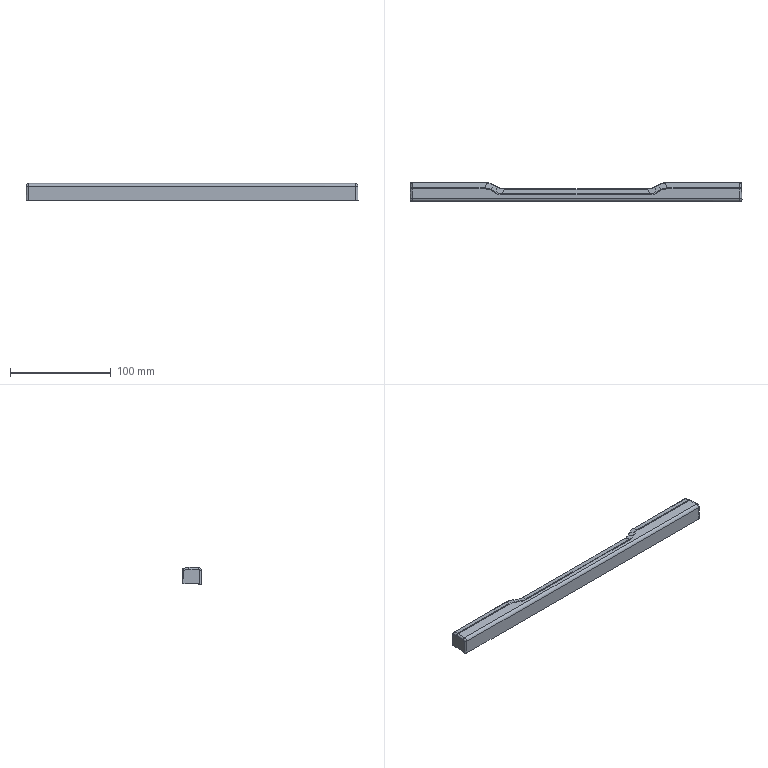Part | STEP file | 5091206W | 1 solid | 101 faces | box 329.891 x 19 x 17 mm | volume 29146 mm3 | cylinder 36 | plane 35 | spline 22 | cone 8 | commonest cylinder face diameters 4 x10 1 x7 6 x5 12 x5 2.3 x4 160 x4